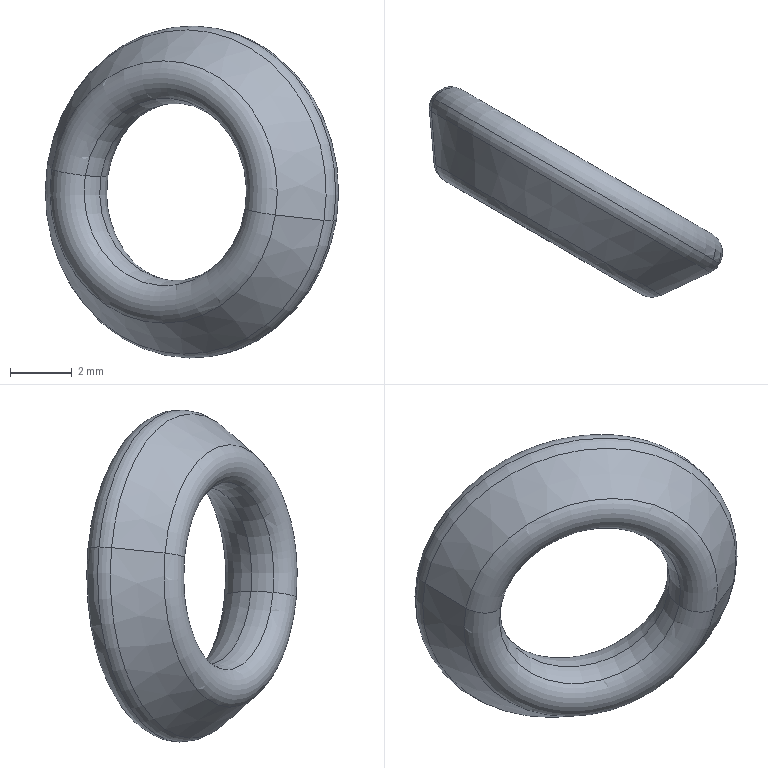Part | SolidWorks | features BaseBody 1 | 1 solid | 12 faces | box 9.466 x 6.792 x 10.714 mm | volume 122.784 mm3 | torus 10 | cone 2